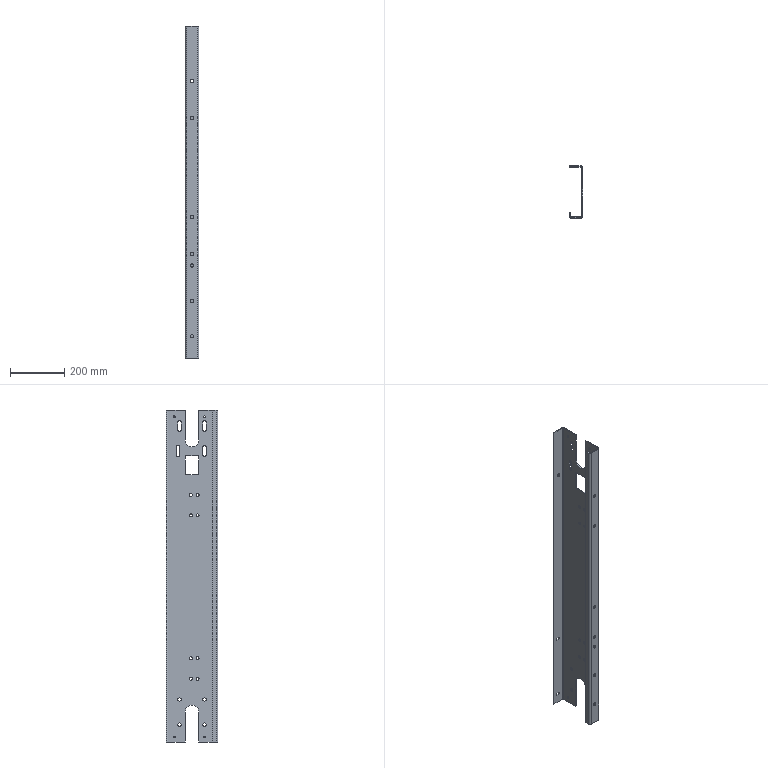Part | STEP file | PN_0040_bent channel_default_machined_ | 1 solid | 111 faces | box 50 x 190 x 1220 mm | volume 1017042 mm3 | cylinder 77 | plane 34 | commonest cylinder face diameters 12 x36 11 x16 7 x12 10 x4 6.4 x3 12.4 x3